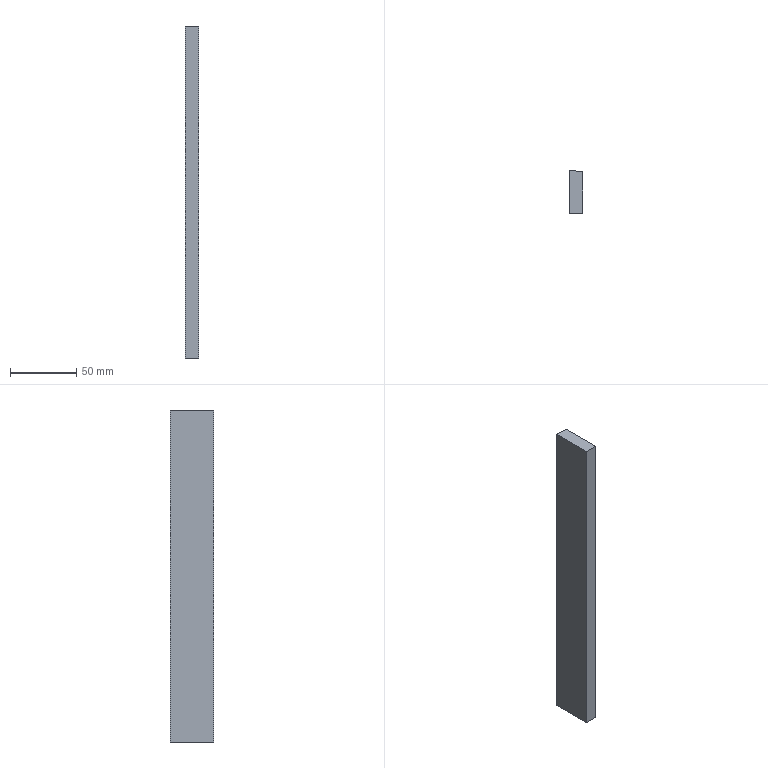Part | SolidWorks | features Extrusion 1 | 1 solid | 6 faces | box 10 x 32.5 x 250 mm | volume 79715 mm3 | plane 6
STEP:
#1=CARTESIAN_POINT('',(0.,0.,0.));
#2=VERTEX_POINT('',#1);
#3=CARTESIAN_POINT('',(10.,0.,0.));
#4=VERTEX_POINT('',#3);
#5=CARTESIAN_POINT('',(0.,0.,0.));
#6=DIRECTION('',(1.,0.,0.));
#7=VECTOR('',#6,1000.);
#8=LINE('',#5,#7);
#9=EDGE_CURVE('',#2,#4,#8,.T.);
#10=ORIENTED_EDGE('',*,*,#9,.T.);
#11=CARTESIAN_POINT('',(10.,0.,250.));
#12=VERTEX_POINT('',#11);
#13=CARTESIAN_POINT('',(10.,0.,250.));
#14=DIRECTION('',(0.,0.,-1.));
#15=VECTOR('',#14,1000.);
#16=LINE('',#13,#15);
#17=EDGE_CURVE('',#12,#4,#16,.T.);
#18=ORIENTED_EDGE('',*,*,#17,.F.);
#19=CARTESIAN_POINT('',(0.,0.,250.));
#20=VERTEX_POINT('',#19);
#21=CARTESIAN_POINT('',(0.,0.,250.));
#22=DIRECTION('',(1.,0.,0.));
#23=VECTOR('',#22,1000.);
#24=LINE('',#21,#23);
#25=EDGE_CURVE('',#20,#12,#24,.T.);
#26=ORIENTED_EDGE('',*,*,#25,.F.);
#27=CARTESIAN_POINT('',(0.,0.,250.));
#28=DIRECTION('',(0.,0.,-1.));
#29=VECTOR('',#28,1000.);
#30=LINE('',#27,#29);
#31=EDGE_CURVE('',#20,#2,#30,.T.);
#32=ORIENTED_EDGE('',*,*,#31,.T.);
#33=EDGE_LOOP('',(#10,#18,#26,#32));
#34=FACE_OUTER_BOUND('',#33,.T.);
#35=CARTESIAN_POINT('',(0.,0.,250.));
#36=DIRECTION('',(0.,1.,0.));
#37=DIRECTION('',(0.,0.,1.));
#38=AXIS2_PLACEMENT_3D('',#35,#36,#37);
#39=PLANE('',#38);
#40=ADVANCED_FACE('',(#34),#39,.F.);
#41=CARTESIAN_POINT('',(10.,31.272,0.));
#42=VERTEX_POINT('',#41);
#43=CARTESIAN_POINT('',(10.,0.,0.));
#44=DIRECTION('',(0.,1.,0.));
#45=VECTOR('',#44,1000.);
#46=LINE('',#43,#45);
#47=EDGE_CURVE('',#4,#42,#46,.T.);
#48=ORIENTED_EDGE('',*,*,#47,.T.);
#49=CARTESIAN_POINT('',(10.,31.272,250.));
#50=VERTEX_POINT('',#49);
#51=CARTESIAN_POINT('',(10.,31.272,250.));
#52=DIRECTION('',(0.,0.,-1.));
#53=VECTOR('',#52,1000.);
#54=LINE('',#51,#53);
#55=EDGE_CURVE('',#50,#42,#54,.T.);
#56=ORIENTED_EDGE('',*,*,#55,.F.);
#57=CARTESIAN_POINT('',(10.,0.,250.));
#58=DIRECTION('',(0.,1.,0.));
#59=VECTOR('',#58,1000.);
#60=LINE('',#57,#59);
#61=EDGE_CURVE('',#12,#50,#60,.T.);
#62=ORIENTED_EDGE('',*,*,#61,.F.);
#63=ORIENTED_EDGE('',*,*,#17,.T.);
#64=EDGE_LOOP('',(#48,#56,#62,#63));
#65=FACE_OUTER_BOUND('',#64,.T.);
#66=CARTESIAN_POINT('',(10.,0.,250.));
#67=DIRECTION('',(-1.,0.,0.));
#68=DIRECTION('',(0.,0.,1.));
#69=AXIS2_PLACEMENT_3D('',#66,#67,#68);
#70=PLANE('',#69);
#71=ADVANCED_FACE('',(#65),#70,.F.);
#72=CARTESIAN_POINT('',(0.,32.5,0.));
#73=VERTEX_POINT('',#72);
#74=CARTESIAN_POINT('',(10.,31.272,0.));
#75=DIRECTION('',(-0.9925,0.1219,0.));
#76=VECTOR('',#75,1000.);
#77=LINE('',#74,#76);
#78=EDGE_CURVE('',#42,#73,#77,.T.);
#79=ORIENTED_EDGE('',*,*,#78,.T.);
#80=CARTESIAN_POINT('',(0.,32.5,250.));
#81=VERTEX_POINT('',#80);
#82=CARTESIAN_POINT('',(0.,32.5,250.));
#83=DIRECTION('',(0.,0.,-1.));
#84=VECTOR('',#83,1000.);
#85=LINE('',#82,#84);
#86=EDGE_CURVE('',#81,#73,#85,.T.);
#87=ORIENTED_EDGE('',*,*,#86,.F.);
#88=CARTESIAN_POINT('',(10.,31.272,250.));
#89=DIRECTION('',(-0.9925,0.1219,0.));
#90=VECTOR('',#89,1000.);
#91=LINE('',#88,#90);
#92=EDGE_CURVE('',#50,#81,#91,.T.);
#93=ORIENTED_EDGE('',*,*,#92,.F.);
#94=ORIENTED_EDGE('',*,*,#55,.T.);
#95=EDGE_LOOP('',(#79,#87,#93,#94));
#96=FACE_OUTER_BOUND('',#95,.T.);
#97=CARTESIAN_POINT('',(10.,31.272,250.));
#98=DIRECTION('',(-0.1219,-0.9925,0.));
#99=DIRECTION('',(0.9925,-0.1219,0.));
#100=AXIS2_PLACEMENT_3D('',#97,#98,#99);
#101=PLANE('',#100);
#102=ADVANCED_FACE('',(#96),#101,.F.);
#103=CARTESIAN_POINT('',(0.,0.,0.));
#104=DIRECTION('',(0.,-1.,0.));
#105=VECTOR('',#104,1000.);
#106=LINE('',#103,#105);
#107=EDGE_CURVE('',#73,#2,#106,.T.);
#108=ORIENTED_EDGE('',*,*,#107,.T.);
#109=ORIENTED_EDGE('',*,*,#31,.F.);
#110=CARTESIAN_POINT('',(0.,0.,250.));
#111=DIRECTION('',(0.,-1.,0.));
#112=VECTOR('',#111,1000.);
#113=LINE('',#110,#112);
#114=EDGE_CURVE('',#81,#20,#113,.T.);
#115=ORIENTED_EDGE('',*,*,#114,.F.);
#116=ORIENTED_EDGE('',*,*,#86,.T.);
#117=EDGE_LOOP('',(#108,#109,#115,#116));
#118=FACE_OUTER_BOUND('',#117,.T.);
#119=CARTESIAN_POINT('',(0.,0.,250.));
#120=DIRECTION('',(1.,0.,0.));
#121=DIRECTION('',(0.,0.,-1.));
#122=AXIS2_PLACEMENT_3D('',#119,#120,#121);
#123=PLANE('',#122);
#124=ADVANCED_FACE('',(#118),#123,.F.);
#125=ORIENTED_EDGE('',*,*,#25,.T.);
#126=ORIENTED_EDGE('',*,*,#61,.T.);
#127=ORIENTED_EDGE('',*,*,#92,.T.);
#128=ORIENTED_EDGE('',*,*,#114,.T.);
#129=EDGE_LOOP('',(#125,#126,#127,#128));
#130=FACE_OUTER_BOUND('',#129,.T.);
#131=CARTESIAN_POINT('',(0.,0.,250.));
#132=DIRECTION('',(0.,0.,1.));
#133=DIRECTION('',(1.,0.,0.));
#134=AXIS2_PLACEMENT_3D('',#131,#132,#133);
#135=PLANE('',#134);
#136=ADVANCED_FACE('',(#130),#135,.T.);
#137=ORIENTED_EDGE('',*,*,#9,.F.);
#138=ORIENTED_EDGE('',*,*,#107,.F.);
#139=ORIENTED_EDGE('',*,*,#78,.F.);
#140=ORIENTED_EDGE('',*,*,#47,.F.);
#141=EDGE_LOOP('',(#137,#138,#139,#140));
#142=FACE_OUTER_BOUND('',#141,.T.);
#143=CARTESIAN_POINT('',(0.,0.,0.));
#144=DIRECTION('',(0.,0.,1.));
#145=DIRECTION('',(1.,0.,0.));
#146=AXIS2_PLACEMENT_3D('',#143,#144,#145);
#147=PLANE('',#146);
#148=ADVANCED_FACE('',(#142),#147,.F.);
#149=CLOSED_SHELL('',(#40,#71,#102,#124,#136,#148));
#150=MANIFOLD_SOLID_BREP('',#149);
#151=CARTESIAN_POINT('',(0.,0.,0.));
#152=DIRECTION('',(0.,0.,1.));
#153=DIRECTION('',(1.,0.,0.));
#154=AXIS2_PLACEMENT_3D('',#151,#152,#153);
#155=(LENGTH_UNIT()NAMED_UNIT(*)SI_UNIT(.MILLI.,.METRE.));
#156=UNCERTAINTY_MEASURE_WITH_UNIT(LENGTH_MEASURE(0.00001),#155,'','');
#157=(NAMED_UNIT(*)PLANE_ANGLE_UNIT()SI_UNIT($,.RADIAN.));
#158=(NAMED_UNIT(*)SI_UNIT($,.STERADIAN.)SOLID_ANGLE_UNIT());
#159=(GEOMETRIC_REPRESENTATION_CONTEXT(3)GLOBAL_UNCERTAINTY_ASSIGNED_CONTEXT((#156))GLOBAL_UNIT_ASSIGNED_CONTEXT((#155,#157,#158))REPRESENTATION_CONTEXT('',''));
#160=ADVANCED_BREP_SHAPE_REPRESENTATION('',(#150,#154),#159);